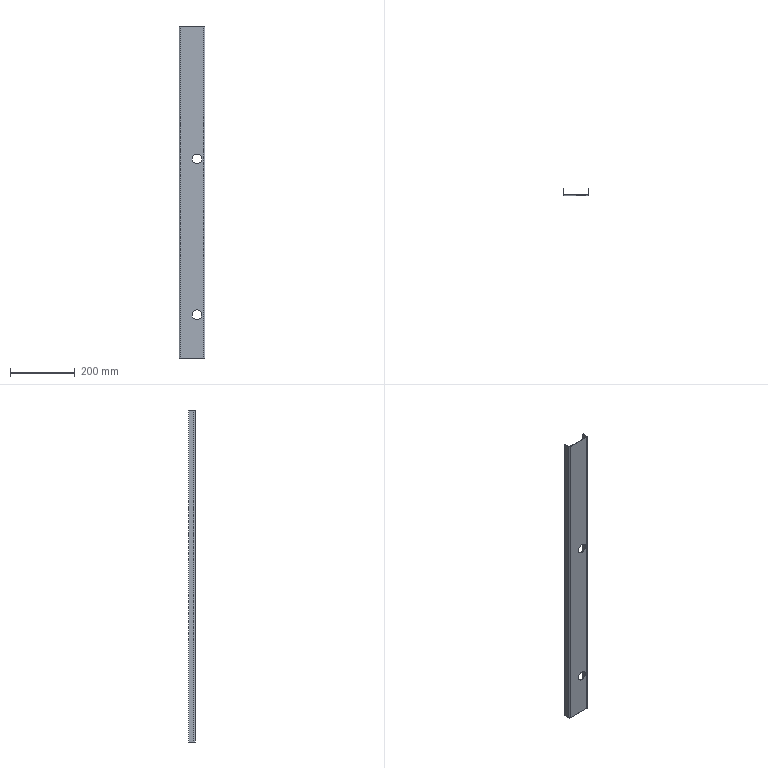Part | NX | features solid 2 | 1 solid | 18 faces | box 80 x 20 x 1022 mm | volume 229013 mm3 | plane 10 | cylinder 8 | commonest cylinder face diameters 30 x4 4 x2 8 x2
STEP:
#1=CARTESIAN_POINT('',(620.,-20.,135.));
#2=VERTEX_POINT('',#1);
#3=CARTESIAN_POINT('',(620.,-22.,135.));
#4=VERTEX_POINT('',#3);
#5=CARTESIAN_POINT('',(620.,1003.321,135.));
#6=DIRECTION('',(0.,-1.,0.));
#7=VECTOR('',#6,1000.);
#8=LINE('',#5,#7);
#9=EDGE_CURVE('',#2,#4,#8,.T.);
#10=ORIENTED_EDGE('',*,*,#9,.F.);
#11=CARTESIAN_POINT('',(650.,-20.,135.));
#12=VERTEX_POINT('',#11);
#13=CARTESIAN_POINT('',(635.,-20.,135.));
#14=DIRECTION('',(0.,1.,0.));
#15=DIRECTION('',(-1.,0.,0.));
#16=AXIS2_PLACEMENT_3D('',#13,#14,#15);
#17=CIRCLE('',#16,15.);
#18=EDGE_CURVE('',#2,#12,#17,.T.);
#19=ORIENTED_EDGE('',*,*,#18,.T.);
#20=CARTESIAN_POINT('',(650.,-22.,135.));
#21=VERTEX_POINT('',#20);
#22=CARTESIAN_POINT('',(650.,1003.321,135.));
#23=DIRECTION('',(0.,-1.,0.));
#24=VECTOR('',#23,1000.);
#25=LINE('',#22,#24);
#26=EDGE_CURVE('',#21,#12,#25,.F.);
#27=ORIENTED_EDGE('',*,*,#26,.F.);
#28=CARTESIAN_POINT('',(635.,-22.,135.));
#29=DIRECTION('',(0.,-1.,0.));
#30=DIRECTION('',(0.,0.,1.));
#31=AXIS2_PLACEMENT_3D('',#28,#29,#30);
#32=CIRCLE('',#31,15.);
#33=EDGE_CURVE('',#21,#4,#32,.T.);
#34=ORIENTED_EDGE('',*,*,#33,.T.);
#35=EDGE_LOOP('',(#10,#19,#27,#34));
#36=FACE_BOUND('',#35,.T.);
#37=CARTESIAN_POINT('',(635.,1003.321,135.));
#38=DIRECTION('',(0.,-1.,0.));
#39=DIRECTION('',(1.,0.,0.));
#40=AXIS2_PLACEMENT_3D('',#37,#38,#39);
#41=CYLINDRICAL_SURFACE('',#40,15.);
#42=ADVANCED_FACE('',(#36),#41,.F.);
#43=CARTESIAN_POINT('',(620.,-22.,615.));
#44=VERTEX_POINT('',#43);
#45=CARTESIAN_POINT('',(620.,-20.,615.));
#46=VERTEX_POINT('',#45);
#47=CARTESIAN_POINT('',(620.,1003.321,615.));
#48=DIRECTION('',(0.,-1.,0.));
#49=VECTOR('',#48,1000.);
#50=LINE('',#47,#49);
#51=EDGE_CURVE('',#44,#46,#50,.F.);
#52=ORIENTED_EDGE('',*,*,#51,.T.);
#53=CARTESIAN_POINT('',(650.,-20.,615.));
#54=VERTEX_POINT('',#53);
#55=CARTESIAN_POINT('',(635.,-20.,615.));
#56=DIRECTION('',(0.,1.,0.));
#57=DIRECTION('',(-1.,0.,0.));
#58=AXIS2_PLACEMENT_3D('',#55,#56,#57);
#59=CIRCLE('',#58,15.);
#60=EDGE_CURVE('',#46,#54,#59,.T.);
#61=ORIENTED_EDGE('',*,*,#60,.T.);
#62=CARTESIAN_POINT('',(650.,-22.,615.));
#63=VERTEX_POINT('',#62);
#64=CARTESIAN_POINT('',(650.,1003.321,615.));
#65=DIRECTION('',(0.,-1.,0.));
#66=VECTOR('',#65,1000.);
#67=LINE('',#64,#66);
#68=EDGE_CURVE('',#54,#63,#67,.T.);
#69=ORIENTED_EDGE('',*,*,#68,.T.);
#70=CARTESIAN_POINT('',(635.,-22.,615.));
#71=DIRECTION('',(0.,-1.,0.));
#72=DIRECTION('',(0.,0.,1.));
#73=AXIS2_PLACEMENT_3D('',#70,#71,#72);
#74=CIRCLE('',#73,15.);
#75=EDGE_CURVE('',#63,#44,#74,.T.);
#76=ORIENTED_EDGE('',*,*,#75,.T.);
#77=EDGE_LOOP('',(#52,#61,#69,#76));
#78=FACE_BOUND('',#77,.T.);
#79=CARTESIAN_POINT('',(635.,1003.321,615.));
#80=DIRECTION('',(0.,-1.,0.));
#81=DIRECTION('',(1.,0.,0.));
#82=AXIS2_PLACEMENT_3D('',#79,#80,#81);
#83=CYLINDRICAL_SURFACE('',#82,15.);
#84=ADVANCED_FACE('',(#78),#83,.F.);
#85=CARTESIAN_POINT('',(660.,-18.,2.));
#86=VERTEX_POINT('',#85);
#87=CARTESIAN_POINT('',(660.,-2.,2.));
#88=VERTEX_POINT('',#87);
#89=CARTESIAN_POINT('',(660.,-22.,2.));
#90=DIRECTION('',(0.,1.,0.));
#91=VECTOR('',#90,1000.);
#92=LINE('',#89,#91);
#93=EDGE_CURVE('',#86,#88,#92,.T.);
#94=ORIENTED_EDGE('',*,*,#93,.T.);
#95=CARTESIAN_POINT('',(660.,-2.,1024.));
#96=VERTEX_POINT('',#95);
#97=CARTESIAN_POINT('',(660.,-2.,1024.));
#98=DIRECTION('',(0.,0.,-1.));
#99=VECTOR('',#98,1000.);
#100=LINE('',#97,#99);
#101=EDGE_CURVE('',#96,#88,#100,.T.);
#102=ORIENTED_EDGE('',*,*,#101,.F.);
#103=CARTESIAN_POINT('',(660.,-18.,1024.));
#104=VERTEX_POINT('',#103);
#105=CARTESIAN_POINT('',(660.,-22.,1024.));
#106=DIRECTION('',(0.,1.,0.));
#107=VECTOR('',#106,1000.);
#108=LINE('',#105,#107);
#109=EDGE_CURVE('',#104,#96,#108,.T.);
#110=ORIENTED_EDGE('',*,*,#109,.F.);
#111=CARTESIAN_POINT('',(660.,-18.,1024.));
#112=DIRECTION('',(0.,0.,-1.));
#113=VECTOR('',#112,1000.);
#114=LINE('',#111,#113);
#115=EDGE_CURVE('',#104,#86,#114,.T.);
#116=ORIENTED_EDGE('',*,*,#115,.T.);
#117=EDGE_LOOP('',(#94,#102,#110,#116));
#118=FACE_BOUND('',#117,.T.);
#119=CARTESIAN_POINT('',(660.,-22.,1024.));
#120=DIRECTION('',(-1.,0.,0.));
#121=DIRECTION('',(0.,1.,0.));
#122=AXIS2_PLACEMENT_3D('',#119,#120,#121);
#123=PLANE('',#122);
#124=ADVANCED_FACE('',(#118),#123,.F.);
#125=CARTESIAN_POINT('',(656.,-22.,2.));
#126=VERTEX_POINT('',#125);
#127=CARTESIAN_POINT('',(656.,-18.,2.));
#128=DIRECTION('',(0.,0.,1.));
#129=DIRECTION('',(0.,1.,0.));
#130=AXIS2_PLACEMENT_3D('',#127,#128,#129);
#131=CIRCLE('',#130,4.);
#132=EDGE_CURVE('',#126,#86,#131,.T.);
#133=ORIENTED_EDGE('',*,*,#132,.T.);
#134=ORIENTED_EDGE('',*,*,#115,.F.);
#135=CARTESIAN_POINT('',(656.,-22.,1024.));
#136=VERTEX_POINT('',#135);
#137=CARTESIAN_POINT('',(656.,-18.,1024.));
#138=DIRECTION('',(0.,0.,1.));
#139=DIRECTION('',(0.,1.,0.));
#140=AXIS2_PLACEMENT_3D('',#137,#138,#139);
#141=CIRCLE('',#140,4.);
#142=EDGE_CURVE('',#136,#104,#141,.T.);
#143=ORIENTED_EDGE('',*,*,#142,.F.);
#144=CARTESIAN_POINT('',(656.,-22.,1024.));
#145=DIRECTION('',(0.,0.,-1.));
#146=VECTOR('',#145,1000.);
#147=LINE('',#144,#146);
#148=EDGE_CURVE('',#136,#126,#147,.T.);
#149=ORIENTED_EDGE('',*,*,#148,.T.);
#150=EDGE_LOOP('',(#133,#134,#143,#149));
#151=FACE_BOUND('',#150,.T.);
#152=CARTESIAN_POINT('',(656.,-18.,1024.));
#153=DIRECTION('',(0.,0.,-1.));
#154=DIRECTION('',(0.,1.,0.));
#155=AXIS2_PLACEMENT_3D('',#152,#153,#154);
#156=CYLINDRICAL_SURFACE('',#155,4.);
#157=ADVANCED_FACE('',(#151),#156,.T.);
#158=ORIENTED_EDGE('',*,*,#75,.F.);
#159=CARTESIAN_POINT('',(635.,-22.,615.));
#160=DIRECTION('',(0.,-1.,0.));
#161=DIRECTION('',(0.,0.,1.));
#162=AXIS2_PLACEMENT_3D('',#159,#160,#161);
#163=CIRCLE('',#162,15.);
#164=EDGE_CURVE('',#44,#63,#163,.T.);
#165=ORIENTED_EDGE('',*,*,#164,.F.);
#166=EDGE_LOOP('',(#158,#165));
#167=FACE_BOUND('',#166,.T.);
#168=ORIENTED_EDGE('',*,*,#33,.F.);
#169=CARTESIAN_POINT('',(635.,-22.,135.));
#170=DIRECTION('',(0.,-1.,0.));
#171=DIRECTION('',(0.,0.,1.));
#172=AXIS2_PLACEMENT_3D('',#169,#170,#171);
#173=CIRCLE('',#172,15.);
#174=EDGE_CURVE('',#4,#21,#173,.T.);
#175=ORIENTED_EDGE('',*,*,#174,.F.);
#176=EDGE_LOOP('',(#168,#175));
#177=FACE_BOUND('',#176,.T.);
#178=CARTESIAN_POINT('',(584.,-22.,2.));
#179=VERTEX_POINT('',#178);
#180=CARTESIAN_POINT('',(580.,-22.,2.));
#181=DIRECTION('',(1.,0.,0.));
#182=VECTOR('',#181,1000.);
#183=LINE('',#180,#182);
#184=EDGE_CURVE('',#179,#126,#183,.T.);
#185=ORIENTED_EDGE('',*,*,#184,.T.);
#186=ORIENTED_EDGE('',*,*,#148,.F.);
#187=CARTESIAN_POINT('',(584.,-22.,1024.));
#188=VERTEX_POINT('',#187);
#189=CARTESIAN_POINT('',(580.,-22.,1024.));
#190=DIRECTION('',(1.,0.,0.));
#191=VECTOR('',#190,1000.);
#192=LINE('',#189,#191);
#193=EDGE_CURVE('',#188,#136,#192,.T.);
#194=ORIENTED_EDGE('',*,*,#193,.F.);
#195=CARTESIAN_POINT('',(584.,-22.,1024.));
#196=DIRECTION('',(0.,0.,-1.));
#197=VECTOR('',#196,1000.);
#198=LINE('',#195,#197);
#199=EDGE_CURVE('',#188,#179,#198,.T.);
#200=ORIENTED_EDGE('',*,*,#199,.T.);
#201=EDGE_LOOP('',(#185,#186,#194,#200));
#202=FACE_BOUND('',#201,.T.);
#203=CARTESIAN_POINT('',(580.,-22.,1024.));
#204=DIRECTION('',(0.,1.,0.));
#205=DIRECTION('',(0.,0.,-1.));
#206=AXIS2_PLACEMENT_3D('',#203,#204,#205);
#207=PLANE('',#206);
#208=ADVANCED_FACE('',(#167,#177,#202),#207,.F.);
#209=CARTESIAN_POINT('',(580.,-18.,2.));
#210=VERTEX_POINT('',#209);
#211=CARTESIAN_POINT('',(584.,-18.,2.));
#212=DIRECTION('',(0.,0.,1.));
#213=DIRECTION('',(0.,1.,0.));
#214=AXIS2_PLACEMENT_3D('',#211,#212,#213);
#215=CIRCLE('',#214,4.);
#216=EDGE_CURVE('',#210,#179,#215,.T.);
#217=ORIENTED_EDGE('',*,*,#216,.T.);
#218=ORIENTED_EDGE('',*,*,#199,.F.);
#219=CARTESIAN_POINT('',(580.,-18.,1024.));
#220=VERTEX_POINT('',#219);
#221=CARTESIAN_POINT('',(584.,-18.,1024.));
#222=DIRECTION('',(0.,0.,1.));
#223=DIRECTION('',(0.,1.,0.));
#224=AXIS2_PLACEMENT_3D('',#221,#222,#223);
#225=CIRCLE('',#224,4.);
#226=EDGE_CURVE('',#220,#188,#225,.T.);
#227=ORIENTED_EDGE('',*,*,#226,.F.);
#228=CARTESIAN_POINT('',(580.,-18.,1024.));
#229=DIRECTION('',(0.,0.,-1.));
#230=VECTOR('',#229,1000.);
#231=LINE('',#228,#230);
#232=EDGE_CURVE('',#220,#210,#231,.T.);
#233=ORIENTED_EDGE('',*,*,#232,.T.);
#234=EDGE_LOOP('',(#217,#218,#227,#233));
#235=FACE_BOUND('',#234,.T.);
#236=CARTESIAN_POINT('',(584.,-18.,1024.));
#237=DIRECTION('',(0.,0.,-1.));
#238=DIRECTION('',(0.,1.,0.));
#239=AXIS2_PLACEMENT_3D('',#236,#237,#238);
#240=CYLINDRICAL_SURFACE('',#239,4.);
#241=ADVANCED_FACE('',(#235),#240,.T.);
#242=CARTESIAN_POINT('',(580.,-2.,2.));
#243=VERTEX_POINT('',#242);
#244=CARTESIAN_POINT('',(580.,-2.,2.));
#245=DIRECTION('',(0.,-1.,0.));
#246=VECTOR('',#245,1000.);
#247=LINE('',#244,#246);
#248=EDGE_CURVE('',#243,#210,#247,.T.);
#249=ORIENTED_EDGE('',*,*,#248,.T.);
#250=ORIENTED_EDGE('',*,*,#232,.F.);
#251=CARTESIAN_POINT('',(580.,-2.,1024.));
#252=VERTEX_POINT('',#251);
#253=CARTESIAN_POINT('',(580.,-2.,1024.));
#254=DIRECTION('',(0.,-1.,0.));
#255=VECTOR('',#254,1000.);
#256=LINE('',#253,#255);
#257=EDGE_CURVE('',#252,#220,#256,.T.);
#258=ORIENTED_EDGE('',*,*,#257,.F.);
#259=CARTESIAN_POINT('',(580.,-2.,1024.));
#260=DIRECTION('',(0.,0.,-1.));
#261=VECTOR('',#260,1000.);
#262=LINE('',#259,#261);
#263=EDGE_CURVE('',#252,#243,#262,.T.);
#264=ORIENTED_EDGE('',*,*,#263,.T.);
#265=EDGE_LOOP('',(#249,#250,#258,#264));
#266=FACE_BOUND('',#265,.T.);
#267=CARTESIAN_POINT('',(580.,-2.,1024.));
#268=DIRECTION('',(1.,0.,0.));
#269=DIRECTION('',(0.,1.,0.));
#270=AXIS2_PLACEMENT_3D('',#267,#268,#269);
#271=PLANE('',#270);
#272=ADVANCED_FACE('',(#266),#271,.F.);
#273=CARTESIAN_POINT('',(658.,-18.,2.));
#274=VERTEX_POINT('',#273);
#275=CARTESIAN_POINT('',(658.,-2.,2.));
#276=VERTEX_POINT('',#275);
#277=CARTESIAN_POINT('',(658.,-22.,2.));
#278=DIRECTION('',(0.,1.,0.));
#279=VECTOR('',#278,1000.);
#280=LINE('',#277,#279);
#281=EDGE_CURVE('',#274,#276,#280,.T.);
#282=ORIENTED_EDGE('',*,*,#281,.F.);
#283=CARTESIAN_POINT('',(658.,-18.,1024.));
#284=VERTEX_POINT('',#283);
#285=CARTESIAN_POINT('',(658.,-18.,1024.));
#286=DIRECTION('',(0.,0.,-1.));
#287=VECTOR('',#286,1000.);
#288=LINE('',#285,#287);
#289=EDGE_CURVE('',#284,#274,#288,.T.);
#290=ORIENTED_EDGE('',*,*,#289,.F.);
#291=CARTESIAN_POINT('',(658.,-2.,1024.));
#292=VERTEX_POINT('',#291);
#293=CARTESIAN_POINT('',(658.,-22.,1024.));
#294=DIRECTION('',(0.,1.,0.));
#295=VECTOR('',#294,1000.);
#296=LINE('',#293,#295);
#297=EDGE_CURVE('',#284,#292,#296,.T.);
#298=ORIENTED_EDGE('',*,*,#297,.T.);
#299=CARTESIAN_POINT('',(658.,-2.,1024.));
#300=DIRECTION('',(0.,0.,-1.));
#301=VECTOR('',#300,1000.);
#302=LINE('',#299,#301);
#303=EDGE_CURVE('',#292,#276,#302,.T.);
#304=ORIENTED_EDGE('',*,*,#303,.T.);
#305=EDGE_LOOP('',(#282,#290,#298,#304));
#306=FACE_BOUND('',#305,.T.);
#307=CARTESIAN_POINT('',(658.,-22.,1024.));
#308=DIRECTION('',(-1.,0.,0.));
#309=DIRECTION('',(0.,1.,0.));
#310=AXIS2_PLACEMENT_3D('',#307,#308,#309);
#311=PLANE('',#310);
#312=ADVANCED_FACE('',(#306),#311,.T.);
#313=CARTESIAN_POINT('',(656.,-20.,2.));
#314=VERTEX_POINT('',#313);
#315=CARTESIAN_POINT('',(656.,-18.,2.));
#316=DIRECTION('',(0.,0.,1.));
#317=DIRECTION('',(0.,1.,0.));
#318=AXIS2_PLACEMENT_3D('',#315,#316,#317);
#319=CIRCLE('',#318,2.);
#320=EDGE_CURVE('',#314,#274,#319,.T.);
#321=ORIENTED_EDGE('',*,*,#320,.F.);
#322=CARTESIAN_POINT('',(656.,-20.,1024.));
#323=VERTEX_POINT('',#322);
#324=CARTESIAN_POINT('',(656.,-20.,1024.));
#325=DIRECTION('',(0.,0.,-1.));
#326=VECTOR('',#325,1000.);
#327=LINE('',#324,#326);
#328=EDGE_CURVE('',#323,#314,#327,.T.);
#329=ORIENTED_EDGE('',*,*,#328,.F.);
#330=CARTESIAN_POINT('',(656.,-18.,1024.));
#331=DIRECTION('',(0.,0.,1.));
#332=DIRECTION('',(0.,1.,0.));
#333=AXIS2_PLACEMENT_3D('',#330,#331,#332);
#334=CIRCLE('',#333,2.);
#335=EDGE_CURVE('',#323,#284,#334,.T.);
#336=ORIENTED_EDGE('',*,*,#335,.T.);
#337=ORIENTED_EDGE('',*,*,#289,.T.);
#338=EDGE_LOOP('',(#321,#329,#336,#337));
#339=FACE_BOUND('',#338,.T.);
#340=CARTESIAN_POINT('',(656.,-18.,1024.));
#341=DIRECTION('',(0.,0.,-1.));
#342=DIRECTION('',(0.,1.,0.));
#343=AXIS2_PLACEMENT_3D('',#340,#341,#342);
#344=CYLINDRICAL_SURFACE('',#343,2.);
#345=ADVANCED_FACE('',(#339),#344,.F.);
#346=CARTESIAN_POINT('',(635.,-20.,615.));
#347=DIRECTION('',(0.,1.,0.));
#348=DIRECTION('',(-1.,0.,0.));
#349=AXIS2_PLACEMENT_3D('',#346,#347,#348);
#350=CIRCLE('',#349,15.);
#351=EDGE_CURVE('',#54,#46,#350,.T.);
#352=ORIENTED_EDGE('',*,*,#351,.F.);
#353=ORIENTED_EDGE('',*,*,#60,.F.);
#354=EDGE_LOOP('',(#352,#353));
#355=FACE_BOUND('',#354,.T.);
#356=CARTESIAN_POINT('',(635.,-20.,135.));
#357=DIRECTION('',(0.,1.,0.));
#358=DIRECTION('',(-1.,0.,0.));
#359=AXIS2_PLACEMENT_3D('',#356,#357,#358);
#360=CIRCLE('',#359,15.);
#361=EDGE_CURVE('',#12,#2,#360,.T.);
#362=ORIENTED_EDGE('',*,*,#361,.F.);
#363=ORIENTED_EDGE('',*,*,#18,.F.);
#364=EDGE_LOOP('',(#362,#363));
#365=FACE_BOUND('',#364,.T.);
#366=CARTESIAN_POINT('',(584.,-20.,2.));
#367=VERTEX_POINT('',#366);
#368=CARTESIAN_POINT('',(580.,-20.,2.));
#369=DIRECTION('',(1.,0.,0.));
#370=VECTOR('',#369,1000.);
#371=LINE('',#368,#370);
#372=EDGE_CURVE('',#367,#314,#371,.T.);
#373=ORIENTED_EDGE('',*,*,#372,.F.);
#374=CARTESIAN_POINT('',(584.,-20.,1024.));
#375=VERTEX_POINT('',#374);
#376=CARTESIAN_POINT('',(584.,-20.,1024.));
#377=DIRECTION('',(0.,0.,-1.));
#378=VECTOR('',#377,1000.);
#379=LINE('',#376,#378);
#380=EDGE_CURVE('',#375,#367,#379,.T.);
#381=ORIENTED_EDGE('',*,*,#380,.F.);
#382=CARTESIAN_POINT('',(580.,-20.,1024.));
#383=DIRECTION('',(1.,0.,0.));
#384=VECTOR('',#383,1000.);
#385=LINE('',#382,#384);
#386=EDGE_CURVE('',#375,#323,#385,.T.);
#387=ORIENTED_EDGE('',*,*,#386,.T.);
#388=ORIENTED_EDGE('',*,*,#328,.T.);
#389=EDGE_LOOP('',(#373,#381,#387,#388));
#390=FACE_BOUND('',#389,.T.);
#391=CARTESIAN_POINT('',(580.,-20.,1024.));
#392=DIRECTION('',(0.,1.,0.));
#393=DIRECTION('',(0.,0.,-1.));
#394=AXIS2_PLACEMENT_3D('',#391,#392,#393);
#395=PLANE('',#394);
#396=ADVANCED_FACE('',(#355,#365,#390),#395,.T.);
#397=CARTESIAN_POINT('',(582.,-18.,2.));
#398=VERTEX_POINT('',#397);
#399=CARTESIAN_POINT('',(584.,-18.,2.));
#400=DIRECTION('',(0.,0.,1.));
#401=DIRECTION('',(0.,1.,0.));
#402=AXIS2_PLACEMENT_3D('',#399,#400,#401);
#403=CIRCLE('',#402,2.);
#404=EDGE_CURVE('',#398,#367,#403,.T.);
#405=ORIENTED_EDGE('',*,*,#404,.F.);
#406=CARTESIAN_POINT('',(582.,-18.,1024.));
#407=VERTEX_POINT('',#406);
#408=CARTESIAN_POINT('',(582.,-18.,1024.));
#409=DIRECTION('',(0.,0.,-1.));
#410=VECTOR('',#409,1000.);
#411=LINE('',#408,#410);
#412=EDGE_CURVE('',#407,#398,#411,.T.);
#413=ORIENTED_EDGE('',*,*,#412,.F.);
#414=CARTESIAN_POINT('',(584.,-18.,1024.));
#415=DIRECTION('',(0.,0.,1.));
#416=DIRECTION('',(0.,1.,0.));
#417=AXIS2_PLACEMENT_3D('',#414,#415,#416);
#418=CIRCLE('',#417,2.);
#419=EDGE_CURVE('',#407,#375,#418,.T.);
#420=ORIENTED_EDGE('',*,*,#419,.T.);
#421=ORIENTED_EDGE('',*,*,#380,.T.);
#422=EDGE_LOOP('',(#405,#413,#420,#421));
#423=FACE_BOUND('',#422,.T.);
#424=CARTESIAN_POINT('',(584.,-18.,1024.));
#425=DIRECTION('',(0.,0.,-1.));
#426=DIRECTION('',(0.,1.,0.));
#427=AXIS2_PLACEMENT_3D('',#424,#425,#426);
#428=CYLINDRICAL_SURFACE('',#427,2.);
#429=ADVANCED_FACE('',(#423),#428,.F.);
#430=CARTESIAN_POINT('',(582.,-2.,2.));
#431=VERTEX_POINT('',#430);
#432=CARTESIAN_POINT('',(582.,-2.,2.));
#433=DIRECTION('',(0.,-1.,0.));
#434=VECTOR('',#433,1000.);
#435=LINE('',#432,#434);
#436=EDGE_CURVE('',#431,#398,#435,.T.);
#437=ORIENTED_EDGE('',*,*,#436,.F.);
#438=CARTESIAN_POINT('',(582.,-2.,1024.));
#439=VERTEX_POINT('',#438);
#440=CARTESIAN_POINT('',(582.,-2.,1024.));
#441=DIRECTION('',(0.,0.,-1.));
#442=VECTOR('',#441,1000.);
#443=LINE('',#440,#442);
#444=EDGE_CURVE('',#439,#431,#443,.T.);
#445=ORIENTED_EDGE('',*,*,#444,.F.);
#446=CARTESIAN_POINT('',(582.,-2.,1024.));
#447=DIRECTION('',(0.,-1.,0.));
#448=VECTOR('',#447,1000.);
#449=LINE('',#446,#448);
#450=EDGE_CURVE('',#439,#407,#449,.T.);
#451=ORIENTED_EDGE('',*,*,#450,.T.);
#452=ORIENTED_EDGE('',*,*,#412,.T.);
#453=EDGE_LOOP('',(#437,#445,#451,#452));
#454=FACE_BOUND('',#453,.T.);
#455=CARTESIAN_POINT('',(582.,-2.,1024.));
#456=DIRECTION('',(1.,0.,0.));
#457=DIRECTION('',(0.,1.,0.));
#458=AXIS2_PLACEMENT_3D('',#455,#456,#457);
#459=PLANE('',#458);
#460=ADVANCED_FACE('',(#454),#459,.T.);
#461=ORIENTED_EDGE('',*,*,#263,.F.);
#462=CARTESIAN_POINT('',(580.,-2.,1024.));
#463=DIRECTION('',(1.,0.,0.));
#464=VECTOR('',#463,1000.);
#465=LINE('',#462,#464);
#466=EDGE_CURVE('',#252,#439,#465,.T.);
#467=ORIENTED_EDGE('',*,*,#466,.T.);
#468=ORIENTED_EDGE('',*,*,#444,.T.);
#469=CARTESIAN_POINT('',(580.,-2.,2.));
#470=DIRECTION('',(1.,0.,0.));
#471=VECTOR('',#470,1000.);
#472=LINE('',#469,#471);
#473=EDGE_CURVE('',#243,#431,#472,.T.);
#474=ORIENTED_EDGE('',*,*,#473,.F.);
#475=EDGE_LOOP('',(#461,#467,#468,#474));
#476=FACE_BOUND('',#475,.T.);
#477=CARTESIAN_POINT('',(580.,-2.,1024.));
#478=DIRECTION('',(0.,-1.,0.));
#479=DIRECTION('',(-1.,0.,0.));
#480=AXIS2_PLACEMENT_3D('',#477,#478,#479);
#481=PLANE('',#480);
#482=ADVANCED_FACE('',(#476),#481,.F.);
#483=ORIENTED_EDGE('',*,*,#436,.T.);
#484=ORIENTED_EDGE('',*,*,#404,.T.);
#485=ORIENTED_EDGE('',*,*,#372,.T.);
#486=ORIENTED_EDGE('',*,*,#320,.T.);
#487=ORIENTED_EDGE('',*,*,#281,.T.);
#488=CARTESIAN_POINT('',(660.,-2.,2.));
#489=DIRECTION('',(-1.,0.,0.));
#490=VECTOR('',#489,1000.);
#491=LINE('',#488,#490);
#492=EDGE_CURVE('',#88,#276,#491,.T.);
#493=ORIENTED_EDGE('',*,*,#492,.F.);
#494=ORIENTED_EDGE('',*,*,#93,.F.);
#495=ORIENTED_EDGE('',*,*,#132,.F.);
#496=ORIENTED_EDGE('',*,*,#184,.F.);
#497=ORIENTED_EDGE('',*,*,#216,.F.);
#498=ORIENTED_EDGE('',*,*,#248,.F.);
#499=ORIENTED_EDGE('',*,*,#473,.T.);
#500=EDGE_LOOP('',(#483,#484,#485,#486,#487,#493,#494,#495,#496,#497,#498,#499));
#501=FACE_BOUND('',#500,.T.);
#502=CARTESIAN_POINT('',(580.,-2.,2.));
#503=DIRECTION('',(0.,0.,1.));
#504=DIRECTION('',(0.,-1.,0.));
#505=AXIS2_PLACEMENT_3D('',#502,#503,#504);
#506=PLANE('',#505);
#507=ADVANCED_FACE('',(#501),#506,.F.);
#508=CARTESIAN_POINT('',(660.,-2.,1024.));
#509=DIRECTION('',(-1.,0.,0.));
#510=VECTOR('',#509,1000.);
#511=LINE('',#508,#510);
#512=EDGE_CURVE('',#96,#292,#511,.T.);
#513=ORIENTED_EDGE('',*,*,#512,.F.);
#514=ORIENTED_EDGE('',*,*,#101,.T.);
#515=ORIENTED_EDGE('',*,*,#492,.T.);
#516=ORIENTED_EDGE('',*,*,#303,.F.);
#517=EDGE_LOOP('',(#513,#514,#515,#516));
#518=FACE_BOUND('',#517,.T.);
#519=CARTESIAN_POINT('',(660.,-2.,1024.));
#520=DIRECTION('',(0.,1.,0.));
#521=DIRECTION('',(0.,0.,-1.));
#522=AXIS2_PLACEMENT_3D('',#519,#520,#521);
#523=PLANE('',#522);
#524=ADVANCED_FACE('',(#518),#523,.T.);
#525=ORIENTED_EDGE('',*,*,#297,.F.);
#526=ORIENTED_EDGE('',*,*,#335,.F.);
#527=ORIENTED_EDGE('',*,*,#386,.F.);
#528=ORIENTED_EDGE('',*,*,#419,.F.);
#529=ORIENTED_EDGE('',*,*,#450,.F.);
#530=ORIENTED_EDGE('',*,*,#466,.F.);
#531=ORIENTED_EDGE('',*,*,#257,.T.);
#532=ORIENTED_EDGE('',*,*,#226,.T.);
#533=ORIENTED_EDGE('',*,*,#193,.T.);
#534=ORIENTED_EDGE('',*,*,#142,.T.);
#535=ORIENTED_EDGE('',*,*,#109,.T.);
#536=ORIENTED_EDGE('',*,*,#512,.T.);
#537=EDGE_LOOP('',(#525,#526,#527,#528,#529,#530,#531,#532,#533,#534,#535,#536));
#538=FACE_BOUND('',#537,.T.);
#539=CARTESIAN_POINT('',(660.,-22.,1024.));
#540=DIRECTION('',(0.,0.,1.));
#541=DIRECTION('',(0.,-1.,0.));
#542=AXIS2_PLACEMENT_3D('',#539,#540,#541);
#543=PLANE('',#542);
#544=ADVANCED_FACE('',(#538),#543,.T.);
#545=ORIENTED_EDGE('',*,*,#351,.T.);
#546=ORIENTED_EDGE('',*,*,#51,.F.);
#547=ORIENTED_EDGE('',*,*,#164,.T.);
#548=ORIENTED_EDGE('',*,*,#68,.F.);
#549=EDGE_LOOP('',(#545,#546,#547,#548));
#550=FACE_BOUND('',#549,.T.);
#551=CARTESIAN_POINT('',(635.,1003.321,615.));
#552=DIRECTION('',(0.,-1.,0.));
#553=DIRECTION('',(1.,0.,0.));
#554=AXIS2_PLACEMENT_3D('',#551,#552,#553);
#555=CYLINDRICAL_SURFACE('',#554,15.);
#556=ADVANCED_FACE('',(#550),#555,.F.);
#557=ORIENTED_EDGE('',*,*,#361,.T.);
#558=ORIENTED_EDGE('',*,*,#9,.T.);
#559=ORIENTED_EDGE('',*,*,#174,.T.);
#560=ORIENTED_EDGE('',*,*,#26,.T.);
#561=EDGE_LOOP('',(#557,#558,#559,#560));
#562=FACE_BOUND('',#561,.T.);
#563=CARTESIAN_POINT('',(635.,1003.321,135.));
#564=DIRECTION('',(0.,-1.,0.));
#565=DIRECTION('',(1.,0.,0.));
#566=AXIS2_PLACEMENT_3D('',#563,#564,#565);
#567=CYLINDRICAL_SURFACE('',#566,15.);
#568=ADVANCED_FACE('',(#562),#567,.F.);
#569=CLOSED_SHELL('',(#42,#84,#124,#157,#208,#241,#272,#312,#345,#396,#429,#460,#482,#507,#524,#544,#556,#568));
#570=MANIFOLD_SOLID_BREP('',#569);
#571=(LENGTH_UNIT()NAMED_UNIT(*)SI_UNIT(.MILLI.,.METRE.));
#572=UNCERTAINTY_MEASURE_WITH_UNIT(LENGTH_MEASURE(0.00001),#571,'','');
#573=(NAMED_UNIT(*)PLANE_ANGLE_UNIT()SI_UNIT($,.RADIAN.));
#574=(NAMED_UNIT(*)SI_UNIT($,.STERADIAN.)SOLID_ANGLE_UNIT());
#575=(GEOMETRIC_REPRESENTATION_CONTEXT(3)GLOBAL_UNCERTAINTY_ASSIGNED_CONTEXT((#572))GLOBAL_UNIT_ASSIGNED_CONTEXT((#571,#573,#574))REPRESENTATION_CONTEXT('',''));
#576=ADVANCED_BREP_SHAPE_REPRESENTATION('',(#570),#575);